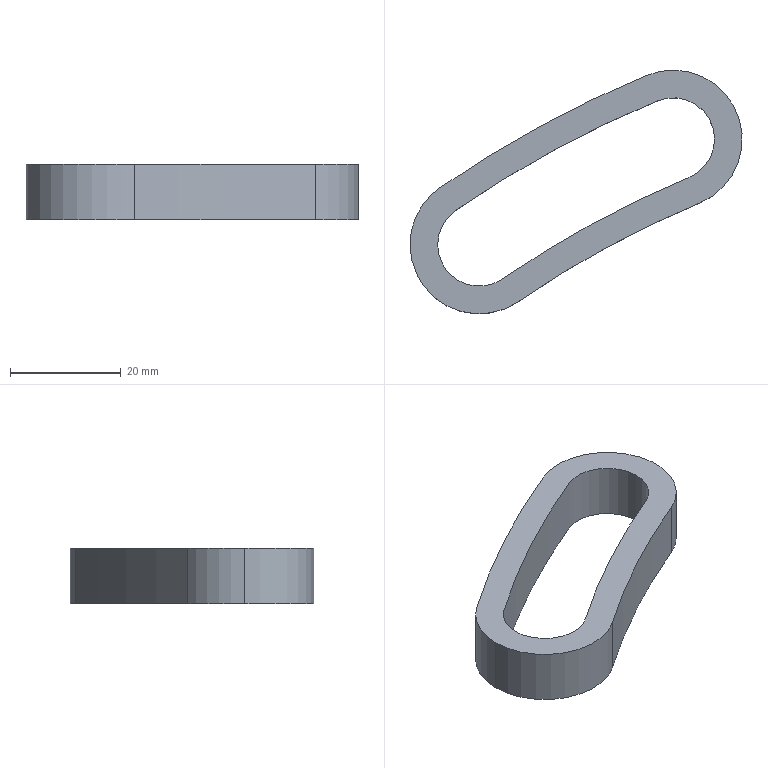Part | SolidWorks | features Extrusion 1 | 1 solid | 12 faces | box 60.075 x 44.074 x 10 mm | volume 7142 mm3 | cylinder 10 | plane 2 | commonest cylinder face diameters 15 x3 25 x3 355 x1 365 x1 395 x1 405 x1
STEP:
#1=CARTESIAN_POINT('',(-403.645,345.362,10.));
#2=VERTEX_POINT('',#1);
#3=CARTESIAN_POINT('',(-406.89,339.186,10.));
#4=VERTEX_POINT('',#3);
#5=CARTESIAN_POINT('',(-399.39,339.186,10.));
#6=DIRECTION('',(0.,0.,1.));
#7=DIRECTION('',(1.,0.,0.));
#8=AXIS2_PLACEMENT_3D('',#5,#6,#7);
#9=CIRCLE('',#8,7.5);
#10=EDGE_CURVE('',#2,#4,#9,.T.);
#11=ORIENTED_EDGE('',*,*,#10,.T.);
#12=CARTESIAN_POINT('',(-406.89,339.186,0.));
#13=VERTEX_POINT('',#12);
#14=CARTESIAN_POINT('',(-406.89,339.186,10.));
#15=DIRECTION('',(0.,0.,-1.));
#16=VECTOR('',#15,1000.);
#17=LINE('',#14,#16);
#18=EDGE_CURVE('',#4,#13,#17,.T.);
#19=ORIENTED_EDGE('',*,*,#18,.T.);
#20=CARTESIAN_POINT('',(-403.645,345.362,0.));
#21=VERTEX_POINT('',#20);
#22=CARTESIAN_POINT('',(-399.39,339.186,0.));
#23=DIRECTION('',(0.,0.,1.));
#24=DIRECTION('',(1.,0.,0.));
#25=AXIS2_PLACEMENT_3D('',#22,#23,#24);
#26=CIRCLE('',#25,7.5);
#27=EDGE_CURVE('',#21,#13,#26,.T.);
#28=ORIENTED_EDGE('',*,*,#27,.F.);
#29=CARTESIAN_POINT('',(-403.645,345.362,10.));
#30=DIRECTION('',(0.,0.,-1.));
#31=VECTOR('',#30,1000.);
#32=LINE('',#29,#31);
#33=EDGE_CURVE('',#2,#21,#32,.T.);
#34=ORIENTED_EDGE('',*,*,#33,.F.);
#35=EDGE_LOOP('',(#11,#19,#28,#34));
#36=FACE_OUTER_BOUND('',#35,.T.);
#37=CARTESIAN_POINT('',(-399.39,339.186,10.));
#38=DIRECTION('',(0.,0.,-1.));
#39=DIRECTION('',(-1.,0.,0.));
#40=AXIS2_PLACEMENT_3D('',#37,#38,#39);
#41=CYLINDRICAL_SURFACE('',#40,7.5);
#42=ADVANCED_FACE('',(#36),#41,.F.);
#43=CARTESIAN_POINT('',(-411.89,339.186,10.));
#44=VERTEX_POINT('',#43);
#45=CARTESIAN_POINT('',(-392.297,328.893,10.));
#46=VERTEX_POINT('',#45);
#47=CARTESIAN_POINT('',(-399.39,339.186,10.));
#48=DIRECTION('',(0.,0.,1.));
#49=DIRECTION('',(1.,0.,0.));
#50=AXIS2_PLACEMENT_3D('',#47,#48,#49);
#51=CIRCLE('',#50,12.5);
#52=EDGE_CURVE('',#44,#46,#51,.T.);
#53=ORIENTED_EDGE('',*,*,#52,.F.);
#54=CARTESIAN_POINT('',(-411.89,339.186,0.));
#55=VERTEX_POINT('',#54);
#56=CARTESIAN_POINT('',(-411.89,339.186,10.));
#57=DIRECTION('',(0.,0.,-1.));
#58=VECTOR('',#57,1000.);
#59=LINE('',#56,#58);
#60=EDGE_CURVE('',#44,#55,#59,.T.);
#61=ORIENTED_EDGE('',*,*,#60,.T.);
#62=CARTESIAN_POINT('',(-392.297,328.893,0.));
#63=VERTEX_POINT('',#62);
#64=CARTESIAN_POINT('',(-399.39,339.186,0.));
#65=DIRECTION('',(0.,0.,1.));
#66=DIRECTION('',(1.,0.,0.));
#67=AXIS2_PLACEMENT_3D('',#64,#65,#66);
#68=CIRCLE('',#67,12.5);
#69=EDGE_CURVE('',#55,#63,#68,.T.);
#70=ORIENTED_EDGE('',*,*,#69,.T.);
#71=CARTESIAN_POINT('',(-392.297,328.893,10.));
#72=DIRECTION('',(0.,0.,-1.));
#73=VECTOR('',#72,1000.);
#74=LINE('',#71,#73);
#75=EDGE_CURVE('',#46,#63,#74,.T.);
#76=ORIENTED_EDGE('',*,*,#75,.F.);
#77=EDGE_LOOP('',(#53,#61,#70,#76));
#78=FACE_OUTER_BOUND('',#77,.T.);
#79=CARTESIAN_POINT('',(-399.39,339.186,10.));
#80=DIRECTION('',(0.,0.,-1.));
#81=DIRECTION('',(-1.,0.,0.));
#82=AXIS2_PLACEMENT_3D('',#79,#80,#81);
#83=CYLINDRICAL_SURFACE('',#82,12.5);
#84=ADVANCED_FACE('',(#78),#83,.T.);
#85=CARTESIAN_POINT('',(-359.529,346.712,10.));
#86=VERTEX_POINT('',#85);
#87=CARTESIAN_POINT('',(-369.099,369.808,10.));
#88=VERTEX_POINT('',#87);
#89=CARTESIAN_POINT('',(-364.314,358.26,10.));
#90=DIRECTION('',(0.,0.,1.));
#91=DIRECTION('',(1.,0.,0.));
#92=AXIS2_PLACEMENT_3D('',#89,#90,#91);
#93=CIRCLE('',#92,12.5);
#94=EDGE_CURVE('',#86,#88,#93,.T.);
#95=ORIENTED_EDGE('',*,*,#94,.T.);
#96=CARTESIAN_POINT('',(-406.482,349.479,10.));
#97=VERTEX_POINT('',#96);
#98=CARTESIAN_POINT('',(-291.585,182.731,10.));
#99=DIRECTION('',(0.,0.,1.));
#100=DIRECTION('',(1.,0.,0.));
#101=AXIS2_PLACEMENT_3D('',#98,#99,#100);
#102=CIRCLE('',#101,202.5);
#103=EDGE_CURVE('',#88,#97,#102,.T.);
#104=ORIENTED_EDGE('',*,*,#103,.T.);
#105=CARTESIAN_POINT('',(-399.39,339.186,10.));
#106=DIRECTION('',(0.,0.,1.));
#107=DIRECTION('',(1.,0.,0.));
#108=AXIS2_PLACEMENT_3D('',#105,#106,#107);
#109=CIRCLE('',#108,12.5);
#110=EDGE_CURVE('',#97,#44,#109,.T.);
#111=ORIENTED_EDGE('',*,*,#110,.T.);
#112=ORIENTED_EDGE('',*,*,#52,.T.);
#113=CARTESIAN_POINT('',(-291.585,182.731,10.));
#114=DIRECTION('',(0.,0.,-1.));
#115=DIRECTION('',(1.,0.,0.));
#116=AXIS2_PLACEMENT_3D('',#113,#114,#115);
#117=CIRCLE('',#116,177.5);
#118=EDGE_CURVE('',#46,#86,#117,.T.);
#119=ORIENTED_EDGE('',*,*,#118,.T.);
#120=EDGE_LOOP('',(#95,#104,#111,#112,#119));
#121=FACE_OUTER_BOUND('',#120,.T.);
#122=CARTESIAN_POINT('',(-367.185,365.189,10.));
#123=VERTEX_POINT('',#122);
#124=CARTESIAN_POINT('',(-291.585,182.731,10.));
#125=DIRECTION('',(0.,0.,1.));
#126=DIRECTION('',(1.,0.,0.));
#127=AXIS2_PLACEMENT_3D('',#124,#125,#126);
#128=CIRCLE('',#127,197.5);
#129=EDGE_CURVE('',#123,#2,#128,.T.);
#130=ORIENTED_EDGE('',*,*,#129,.F.);
#131=CARTESIAN_POINT('',(-361.443,351.331,10.));
#132=VERTEX_POINT('',#131);
#133=CARTESIAN_POINT('',(-364.314,358.26,10.));
#134=DIRECTION('',(0.,0.,1.));
#135=DIRECTION('',(1.,0.,0.));
#136=AXIS2_PLACEMENT_3D('',#133,#134,#135);
#137=CIRCLE('',#136,7.5);
#138=EDGE_CURVE('',#132,#123,#137,.T.);
#139=ORIENTED_EDGE('',*,*,#138,.F.);
#140=CARTESIAN_POINT('',(-395.134,333.01,10.));
#141=VERTEX_POINT('',#140);
#142=CARTESIAN_POINT('',(-291.585,182.731,10.));
#143=DIRECTION('',(0.,0.,-1.));
#144=DIRECTION('',(1.,0.,0.));
#145=AXIS2_PLACEMENT_3D('',#142,#143,#144);
#146=CIRCLE('',#145,182.5);
#147=EDGE_CURVE('',#141,#132,#146,.T.);
#148=ORIENTED_EDGE('',*,*,#147,.F.);
#149=CARTESIAN_POINT('',(-399.39,339.186,10.));
#150=DIRECTION('',(0.,0.,1.));
#151=DIRECTION('',(1.,0.,0.));
#152=AXIS2_PLACEMENT_3D('',#149,#150,#151);
#153=CIRCLE('',#152,7.5);
#154=EDGE_CURVE('',#4,#141,#153,.T.);
#155=ORIENTED_EDGE('',*,*,#154,.F.);
#156=ORIENTED_EDGE('',*,*,#10,.F.);
#157=EDGE_LOOP('',(#130,#139,#148,#155,#156));
#158=FACE_BOUND('',#157,.T.);
#159=CARTESIAN_POINT('',(-327.95,270.495,10.));
#160=DIRECTION('',(0.,0.,1.));
#161=DIRECTION('',(1.,0.,0.));
#162=AXIS2_PLACEMENT_3D('',#159,#160,#161);
#163=PLANE('',#162);
#164=ADVANCED_FACE('',(#121,#158),#163,.T.);
#165=CARTESIAN_POINT('',(-359.529,346.712,0.));
#166=VERTEX_POINT('',#165);
#167=CARTESIAN_POINT('',(-369.099,369.808,0.));
#168=VERTEX_POINT('',#167);
#169=CARTESIAN_POINT('',(-364.314,358.26,0.));
#170=DIRECTION('',(0.,0.,1.));
#171=DIRECTION('',(1.,0.,0.));
#172=AXIS2_PLACEMENT_3D('',#169,#170,#171);
#173=CIRCLE('',#172,12.5);
#174=EDGE_CURVE('',#166,#168,#173,.T.);
#175=ORIENTED_EDGE('',*,*,#174,.F.);
#176=CARTESIAN_POINT('',(-291.585,182.731,0.));
#177=DIRECTION('',(0.,0.,-1.));
#178=DIRECTION('',(1.,0.,0.));
#179=AXIS2_PLACEMENT_3D('',#176,#177,#178);
#180=CIRCLE('',#179,177.5);
#181=EDGE_CURVE('',#63,#166,#180,.T.);
#182=ORIENTED_EDGE('',*,*,#181,.F.);
#183=ORIENTED_EDGE('',*,*,#69,.F.);
#184=CARTESIAN_POINT('',(-406.482,349.479,0.));
#185=VERTEX_POINT('',#184);
#186=CARTESIAN_POINT('',(-399.39,339.186,0.));
#187=DIRECTION('',(0.,0.,1.));
#188=DIRECTION('',(1.,0.,0.));
#189=AXIS2_PLACEMENT_3D('',#186,#187,#188);
#190=CIRCLE('',#189,12.5);
#191=EDGE_CURVE('',#185,#55,#190,.T.);
#192=ORIENTED_EDGE('',*,*,#191,.F.);
#193=CARTESIAN_POINT('',(-291.585,182.731,0.));
#194=DIRECTION('',(0.,0.,1.));
#195=DIRECTION('',(1.,0.,0.));
#196=AXIS2_PLACEMENT_3D('',#193,#194,#195);
#197=CIRCLE('',#196,202.5);
#198=EDGE_CURVE('',#168,#185,#197,.T.);
#199=ORIENTED_EDGE('',*,*,#198,.F.);
#200=EDGE_LOOP('',(#175,#182,#183,#192,#199));
#201=FACE_OUTER_BOUND('',#200,.T.);
#202=CARTESIAN_POINT('',(-361.443,351.331,0.));
#203=VERTEX_POINT('',#202);
#204=CARTESIAN_POINT('',(-367.185,365.189,0.));
#205=VERTEX_POINT('',#204);
#206=CARTESIAN_POINT('',(-364.314,358.26,0.));
#207=DIRECTION('',(0.,0.,1.));
#208=DIRECTION('',(1.,0.,0.));
#209=AXIS2_PLACEMENT_3D('',#206,#207,#208);
#210=CIRCLE('',#209,7.5);
#211=EDGE_CURVE('',#203,#205,#210,.T.);
#212=ORIENTED_EDGE('',*,*,#211,.T.);
#213=CARTESIAN_POINT('',(-291.585,182.731,0.));
#214=DIRECTION('',(0.,0.,1.));
#215=DIRECTION('',(1.,0.,0.));
#216=AXIS2_PLACEMENT_3D('',#213,#214,#215);
#217=CIRCLE('',#216,197.5);
#218=EDGE_CURVE('',#205,#21,#217,.T.);
#219=ORIENTED_EDGE('',*,*,#218,.T.);
#220=ORIENTED_EDGE('',*,*,#27,.T.);
#221=CARTESIAN_POINT('',(-395.134,333.01,0.));
#222=VERTEX_POINT('',#221);
#223=CARTESIAN_POINT('',(-399.39,339.186,0.));
#224=DIRECTION('',(0.,0.,1.));
#225=DIRECTION('',(1.,0.,0.));
#226=AXIS2_PLACEMENT_3D('',#223,#224,#225);
#227=CIRCLE('',#226,7.5);
#228=EDGE_CURVE('',#13,#222,#227,.T.);
#229=ORIENTED_EDGE('',*,*,#228,.T.);
#230=CARTESIAN_POINT('',(-291.585,182.731,0.));
#231=DIRECTION('',(0.,0.,-1.));
#232=DIRECTION('',(1.,0.,0.));
#233=AXIS2_PLACEMENT_3D('',#230,#231,#232);
#234=CIRCLE('',#233,182.5);
#235=EDGE_CURVE('',#222,#203,#234,.T.);
#236=ORIENTED_EDGE('',*,*,#235,.T.);
#237=EDGE_LOOP('',(#212,#219,#220,#229,#236));
#238=FACE_BOUND('',#237,.T.);
#239=CARTESIAN_POINT('',(-327.95,270.495,0.));
#240=DIRECTION('',(0.,0.,1.));
#241=DIRECTION('',(1.,0.,0.));
#242=AXIS2_PLACEMENT_3D('',#239,#240,#241);
#243=PLANE('',#242);
#244=ADVANCED_FACE('',(#201,#238),#243,.F.);
#245=ORIENTED_EDGE('',*,*,#174,.T.);
#246=CARTESIAN_POINT('',(-369.099,369.808,10.));
#247=DIRECTION('',(0.,0.,-1.));
#248=VECTOR('',#247,1000.);
#249=LINE('',#246,#248);
#250=EDGE_CURVE('',#88,#168,#249,.T.);
#251=ORIENTED_EDGE('',*,*,#250,.F.);
#252=ORIENTED_EDGE('',*,*,#94,.F.);
#253=CARTESIAN_POINT('',(-359.529,346.712,10.));
#254=DIRECTION('',(0.,0.,-1.));
#255=VECTOR('',#254,1000.);
#256=LINE('',#253,#255);
#257=EDGE_CURVE('',#86,#166,#256,.T.);
#258=ORIENTED_EDGE('',*,*,#257,.T.);
#259=EDGE_LOOP('',(#245,#251,#252,#258));
#260=FACE_OUTER_BOUND('',#259,.T.);
#261=CARTESIAN_POINT('',(-364.314,358.26,10.));
#262=DIRECTION('',(0.,0.,-1.));
#263=DIRECTION('',(-1.,0.,0.));
#264=AXIS2_PLACEMENT_3D('',#261,#262,#263);
#265=CYLINDRICAL_SURFACE('',#264,12.5);
#266=ADVANCED_FACE('',(#260),#265,.T.);
#267=ORIENTED_EDGE('',*,*,#198,.T.);
#268=CARTESIAN_POINT('',(-406.482,349.479,10.));
#269=DIRECTION('',(0.,0.,-1.));
#270=VECTOR('',#269,1000.);
#271=LINE('',#268,#270);
#272=EDGE_CURVE('',#97,#185,#271,.T.);
#273=ORIENTED_EDGE('',*,*,#272,.F.);
#274=ORIENTED_EDGE('',*,*,#103,.F.);
#275=ORIENTED_EDGE('',*,*,#250,.T.);
#276=EDGE_LOOP('',(#267,#273,#274,#275));
#277=FACE_OUTER_BOUND('',#276,.T.);
#278=CARTESIAN_POINT('',(-291.585,182.731,10.));
#279=DIRECTION('',(0.,0.,-1.));
#280=DIRECTION('',(-1.,0.,0.));
#281=AXIS2_PLACEMENT_3D('',#278,#279,#280);
#282=CYLINDRICAL_SURFACE('',#281,202.5);
#283=ADVANCED_FACE('',(#277),#282,.T.);
#284=ORIENTED_EDGE('',*,*,#60,.F.);
#285=ORIENTED_EDGE('',*,*,#110,.F.);
#286=ORIENTED_EDGE('',*,*,#272,.T.);
#287=ORIENTED_EDGE('',*,*,#191,.T.);
#288=EDGE_LOOP('',(#284,#285,#286,#287));
#289=FACE_OUTER_BOUND('',#288,.T.);
#290=CARTESIAN_POINT('',(-399.39,339.186,10.));
#291=DIRECTION('',(0.,0.,-1.));
#292=DIRECTION('',(-1.,0.,0.));
#293=AXIS2_PLACEMENT_3D('',#290,#291,#292);
#294=CYLINDRICAL_SURFACE('',#293,12.5);
#295=ADVANCED_FACE('',(#289),#294,.T.);
#296=ORIENTED_EDGE('',*,*,#181,.T.);
#297=ORIENTED_EDGE('',*,*,#257,.F.);
#298=ORIENTED_EDGE('',*,*,#118,.F.);
#299=ORIENTED_EDGE('',*,*,#75,.T.);
#300=EDGE_LOOP('',(#296,#297,#298,#299));
#301=FACE_OUTER_BOUND('',#300,.T.);
#302=CARTESIAN_POINT('',(-291.585,182.731,10.));
#303=DIRECTION('',(0.,0.,-1.));
#304=DIRECTION('',(-1.,0.,0.));
#305=AXIS2_PLACEMENT_3D('',#302,#303,#304);
#306=CYLINDRICAL_SURFACE('',#305,177.5);
#307=ADVANCED_FACE('',(#301),#306,.F.);
#308=ORIENTED_EDGE('',*,*,#211,.F.);
#309=CARTESIAN_POINT('',(-361.443,351.331,10.));
#310=DIRECTION('',(0.,0.,-1.));
#311=VECTOR('',#310,1000.);
#312=LINE('',#309,#311);
#313=EDGE_CURVE('',#132,#203,#312,.T.);
#314=ORIENTED_EDGE('',*,*,#313,.F.);
#315=ORIENTED_EDGE('',*,*,#138,.T.);
#316=CARTESIAN_POINT('',(-367.185,365.189,10.));
#317=DIRECTION('',(0.,0.,-1.));
#318=VECTOR('',#317,1000.);
#319=LINE('',#316,#318);
#320=EDGE_CURVE('',#123,#205,#319,.T.);
#321=ORIENTED_EDGE('',*,*,#320,.T.);
#322=EDGE_LOOP('',(#308,#314,#315,#321));
#323=FACE_OUTER_BOUND('',#322,.T.);
#324=CARTESIAN_POINT('',(-364.314,358.26,10.));
#325=DIRECTION('',(0.,0.,-1.));
#326=DIRECTION('',(-1.,0.,0.));
#327=AXIS2_PLACEMENT_3D('',#324,#325,#326);
#328=CYLINDRICAL_SURFACE('',#327,7.5);
#329=ADVANCED_FACE('',(#323),#328,.F.);
#330=ORIENTED_EDGE('',*,*,#218,.F.);
#331=ORIENTED_EDGE('',*,*,#320,.F.);
#332=ORIENTED_EDGE('',*,*,#129,.T.);
#333=ORIENTED_EDGE('',*,*,#33,.T.);
#334=EDGE_LOOP('',(#330,#331,#332,#333));
#335=FACE_OUTER_BOUND('',#334,.T.);
#336=CARTESIAN_POINT('',(-291.585,182.731,10.));
#337=DIRECTION('',(0.,0.,-1.));
#338=DIRECTION('',(-1.,0.,0.));
#339=AXIS2_PLACEMENT_3D('',#336,#337,#338);
#340=CYLINDRICAL_SURFACE('',#339,197.5);
#341=ADVANCED_FACE('',(#335),#340,.F.);
#342=ORIENTED_EDGE('',*,*,#18,.F.);
#343=ORIENTED_EDGE('',*,*,#154,.T.);
#344=CARTESIAN_POINT('',(-395.134,333.01,10.));
#345=DIRECTION('',(0.,0.,-1.));
#346=VECTOR('',#345,1000.);
#347=LINE('',#344,#346);
#348=EDGE_CURVE('',#141,#222,#347,.T.);
#349=ORIENTED_EDGE('',*,*,#348,.T.);
#350=ORIENTED_EDGE('',*,*,#228,.F.);
#351=EDGE_LOOP('',(#342,#343,#349,#350));
#352=FACE_OUTER_BOUND('',#351,.T.);
#353=CARTESIAN_POINT('',(-399.39,339.186,10.));
#354=DIRECTION('',(0.,0.,-1.));
#355=DIRECTION('',(-1.,0.,0.));
#356=AXIS2_PLACEMENT_3D('',#353,#354,#355);
#357=CYLINDRICAL_SURFACE('',#356,7.5);
#358=ADVANCED_FACE('',(#352),#357,.F.);
#359=ORIENTED_EDGE('',*,*,#235,.F.);
#360=ORIENTED_EDGE('',*,*,#348,.F.);
#361=ORIENTED_EDGE('',*,*,#147,.T.);
#362=ORIENTED_EDGE('',*,*,#313,.T.);
#363=EDGE_LOOP('',(#359,#360,#361,#362));
#364=FACE_OUTER_BOUND('',#363,.T.);
#365=CARTESIAN_POINT('',(-291.585,182.731,10.));
#366=DIRECTION('',(0.,0.,-1.));
#367=DIRECTION('',(-1.,0.,0.));
#368=AXIS2_PLACEMENT_3D('',#365,#366,#367);
#369=CYLINDRICAL_SURFACE('',#368,182.5);
#370=ADVANCED_FACE('',(#364),#369,.T.);
#371=CLOSED_SHELL('',(#42,#84,#164,#244,#266,#283,#295,#307,#329,#341,#358,#370));
#372=MANIFOLD_SOLID_BREP('',#371);
#373=CARTESIAN_POINT('',(0.,0.,0.));
#374=DIRECTION('',(0.,0.,1.));
#375=DIRECTION('',(1.,0.,0.));
#376=AXIS2_PLACEMENT_3D('',#373,#374,#375);
#377=(LENGTH_UNIT()NAMED_UNIT(*)SI_UNIT(.MILLI.,.METRE.));
#378=UNCERTAINTY_MEASURE_WITH_UNIT(LENGTH_MEASURE(0.00001),#377,'','');
#379=(NAMED_UNIT(*)PLANE_ANGLE_UNIT()SI_UNIT($,.RADIAN.));
#380=(NAMED_UNIT(*)SI_UNIT($,.STERADIAN.)SOLID_ANGLE_UNIT());
#381=(GEOMETRIC_REPRESENTATION_CONTEXT(3)GLOBAL_UNCERTAINTY_ASSIGNED_CONTEXT((#378))GLOBAL_UNIT_ASSIGNED_CONTEXT((#377,#379,#380))REPRESENTATION_CONTEXT('',''));
#382=ADVANCED_BREP_SHAPE_REPRESENTATION('',(#372,#376),#381);